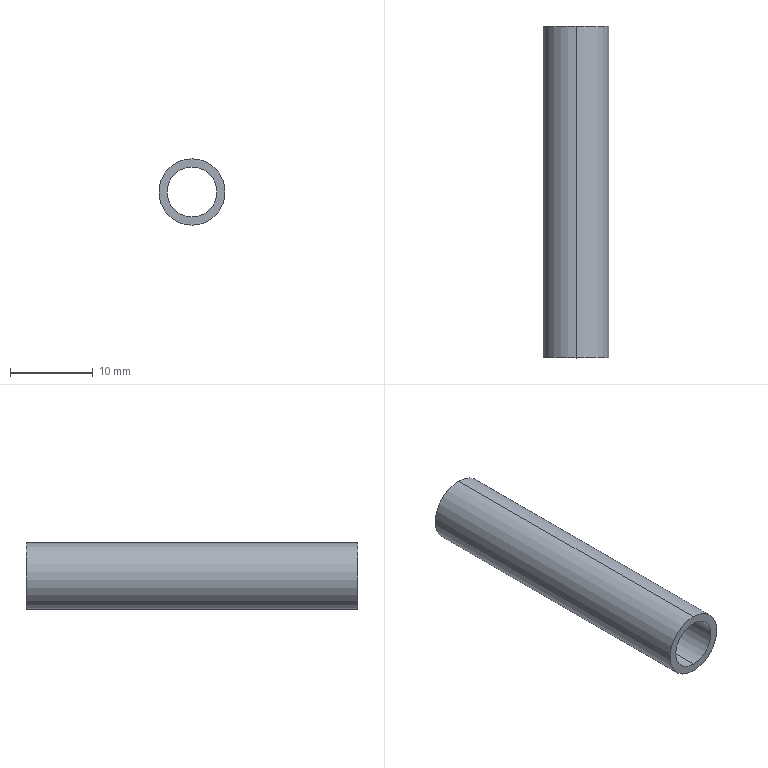Part | SolidWorks | features MirrorStock 1 | 1 solid | 6 faces | box 8 x 40 x 8 mm | volume 879.646 mm3 | cylinder 4 | plane 2 | commonest cylinder face diameters 6 x2 8 x2
STEP:
#1=CARTESIAN_POINT('',(0.,40.,-3.));
#2=VERTEX_POINT('',#1);
#3=CARTESIAN_POINT('',(0.,40.,3.));
#4=VERTEX_POINT('',#3);
#5=CARTESIAN_POINT('',(0.,40.,0.));
#6=DIRECTION('',(0.,-1.,0.));
#7=DIRECTION('',(0.,0.,-1.));
#8=AXIS2_PLACEMENT_3D('',#5,#6,#7);
#9=CIRCLE('',#8,3.);
#10=EDGE_CURVE('',#2,#4,#9,.T.);
#11=ORIENTED_EDGE('',*,*,#10,.F.);
#12=CARTESIAN_POINT('',(0.,0.,-3.));
#13=VERTEX_POINT('',#12);
#14=CARTESIAN_POINT('',(0.,40.,-3.));
#15=DIRECTION('',(0.,-1.,0.));
#16=VECTOR('',#15,1000.);
#17=LINE('',#14,#16);
#18=EDGE_CURVE('',#2,#13,#17,.T.);
#19=ORIENTED_EDGE('',*,*,#18,.T.);
#20=CARTESIAN_POINT('',(0.,0.,3.));
#21=VERTEX_POINT('',#20);
#22=CARTESIAN_POINT('',(0.,0.,0.));
#23=DIRECTION('',(0.,-1.,0.));
#24=DIRECTION('',(0.,0.,-1.));
#25=AXIS2_PLACEMENT_3D('',#22,#23,#24);
#26=CIRCLE('',#25,3.);
#27=EDGE_CURVE('',#13,#21,#26,.T.);
#28=ORIENTED_EDGE('',*,*,#27,.T.);
#29=CARTESIAN_POINT('',(0.,40.,3.));
#30=DIRECTION('',(0.,-1.,0.));
#31=VECTOR('',#30,1000.);
#32=LINE('',#29,#31);
#33=EDGE_CURVE('',#4,#21,#32,.T.);
#34=ORIENTED_EDGE('',*,*,#33,.F.);
#35=EDGE_LOOP('',(#11,#19,#28,#34));
#36=FACE_OUTER_BOUND('',#35,.T.);
#37=CARTESIAN_POINT('',(0.,40.,0.));
#38=DIRECTION('',(0.,-1.,0.));
#39=DIRECTION('',(0.,0.,1.));
#40=AXIS2_PLACEMENT_3D('',#37,#38,#39);
#41=CYLINDRICAL_SURFACE('',#40,3.);
#42=ADVANCED_FACE('',(#36),#41,.F.);
#43=CARTESIAN_POINT('',(0.,40.,4.));
#44=VERTEX_POINT('',#43);
#45=CARTESIAN_POINT('',(0.,40.,-4.));
#46=VERTEX_POINT('',#45);
#47=CARTESIAN_POINT('',(0.,40.,0.));
#48=DIRECTION('',(0.,-1.,0.));
#49=DIRECTION('',(0.,0.,-1.));
#50=AXIS2_PLACEMENT_3D('',#47,#48,#49);
#51=CIRCLE('',#50,4.);
#52=EDGE_CURVE('',#44,#46,#51,.T.);
#53=ORIENTED_EDGE('',*,*,#52,.T.);
#54=CARTESIAN_POINT('',(0.,0.,-4.));
#55=VERTEX_POINT('',#54);
#56=CARTESIAN_POINT('',(0.,40.,-4.));
#57=DIRECTION('',(0.,-1.,0.));
#58=VECTOR('',#57,1000.);
#59=LINE('',#56,#58);
#60=EDGE_CURVE('',#46,#55,#59,.T.);
#61=ORIENTED_EDGE('',*,*,#60,.T.);
#62=CARTESIAN_POINT('',(0.,0.,4.));
#63=VERTEX_POINT('',#62);
#64=CARTESIAN_POINT('',(0.,0.,0.));
#65=DIRECTION('',(0.,-1.,0.));
#66=DIRECTION('',(0.,0.,-1.));
#67=AXIS2_PLACEMENT_3D('',#64,#65,#66);
#68=CIRCLE('',#67,4.);
#69=EDGE_CURVE('',#63,#55,#68,.T.);
#70=ORIENTED_EDGE('',*,*,#69,.F.);
#71=CARTESIAN_POINT('',(0.,40.,4.));
#72=DIRECTION('',(0.,-1.,0.));
#73=VECTOR('',#72,1000.);
#74=LINE('',#71,#73);
#75=EDGE_CURVE('',#44,#63,#74,.T.);
#76=ORIENTED_EDGE('',*,*,#75,.F.);
#77=EDGE_LOOP('',(#53,#61,#70,#76));
#78=FACE_OUTER_BOUND('',#77,.T.);
#79=CARTESIAN_POINT('',(0.,40.,0.));
#80=DIRECTION('',(0.,-1.,0.));
#81=DIRECTION('',(0.,0.,1.));
#82=AXIS2_PLACEMENT_3D('',#79,#80,#81);
#83=CYLINDRICAL_SURFACE('',#82,4.);
#84=ADVANCED_FACE('',(#78),#83,.T.);
#85=ORIENTED_EDGE('',*,*,#52,.F.);
#86=CARTESIAN_POINT('',(0.,40.,0.));
#87=DIRECTION('',(0.,-1.,0.));
#88=DIRECTION('',(0.,0.,-1.));
#89=AXIS2_PLACEMENT_3D('',#86,#87,#88);
#90=CIRCLE('',#89,4.);
#91=EDGE_CURVE('',#46,#44,#90,.T.);
#92=ORIENTED_EDGE('',*,*,#91,.F.);
#93=EDGE_LOOP('',(#85,#92));
#94=FACE_OUTER_BOUND('',#93,.T.);
#95=CARTESIAN_POINT('',(0.,40.,0.));
#96=DIRECTION('',(0.,-1.,0.));
#97=DIRECTION('',(0.,0.,-1.));
#98=AXIS2_PLACEMENT_3D('',#95,#96,#97);
#99=CIRCLE('',#98,3.);
#100=EDGE_CURVE('',#4,#2,#99,.T.);
#101=ORIENTED_EDGE('',*,*,#100,.T.);
#102=ORIENTED_EDGE('',*,*,#10,.T.);
#103=EDGE_LOOP('',(#101,#102));
#104=FACE_BOUND('',#103,.T.);
#105=CARTESIAN_POINT('',(0.,40.,0.));
#106=DIRECTION('',(0.,1.,0.));
#107=DIRECTION('',(0.,0.,-1.));
#108=AXIS2_PLACEMENT_3D('',#105,#106,#107);
#109=PLANE('',#108);
#110=ADVANCED_FACE('',(#94,#104),#109,.T.);
#111=ORIENTED_EDGE('',*,*,#69,.T.);
#112=CARTESIAN_POINT('',(0.,0.,0.));
#113=DIRECTION('',(0.,-1.,0.));
#114=DIRECTION('',(0.,0.,-1.));
#115=AXIS2_PLACEMENT_3D('',#112,#113,#114);
#116=CIRCLE('',#115,4.);
#117=EDGE_CURVE('',#55,#63,#116,.T.);
#118=ORIENTED_EDGE('',*,*,#117,.T.);
#119=EDGE_LOOP('',(#111,#118));
#120=FACE_OUTER_BOUND('',#119,.T.);
#121=CARTESIAN_POINT('',(0.,0.,0.));
#122=DIRECTION('',(0.,-1.,0.));
#123=DIRECTION('',(0.,0.,-1.));
#124=AXIS2_PLACEMENT_3D('',#121,#122,#123);
#125=CIRCLE('',#124,3.);
#126=EDGE_CURVE('',#21,#13,#125,.T.);
#127=ORIENTED_EDGE('',*,*,#126,.F.);
#128=ORIENTED_EDGE('',*,*,#27,.F.);
#129=EDGE_LOOP('',(#127,#128));
#130=FACE_BOUND('',#129,.T.);
#131=CARTESIAN_POINT('',(0.,0.,0.));
#132=DIRECTION('',(0.,1.,0.));
#133=DIRECTION('',(0.,0.,-1.));
#134=AXIS2_PLACEMENT_3D('',#131,#132,#133);
#135=PLANE('',#134);
#136=ADVANCED_FACE('',(#120,#130),#135,.F.);
#137=ORIENTED_EDGE('',*,*,#60,.F.);
#138=ORIENTED_EDGE('',*,*,#91,.T.);
#139=ORIENTED_EDGE('',*,*,#75,.T.);
#140=ORIENTED_EDGE('',*,*,#117,.F.);
#141=EDGE_LOOP('',(#137,#138,#139,#140));
#142=FACE_OUTER_BOUND('',#141,.T.);
#143=CARTESIAN_POINT('',(0.,40.,0.));
#144=DIRECTION('',(0.,-1.,0.));
#145=DIRECTION('',(0.,0.,1.));
#146=AXIS2_PLACEMENT_3D('',#143,#144,#145);
#147=CYLINDRICAL_SURFACE('',#146,4.);
#148=ADVANCED_FACE('',(#142),#147,.T.);
#149=ORIENTED_EDGE('',*,*,#18,.F.);
#150=ORIENTED_EDGE('',*,*,#100,.F.);
#151=ORIENTED_EDGE('',*,*,#33,.T.);
#152=ORIENTED_EDGE('',*,*,#126,.T.);
#153=EDGE_LOOP('',(#149,#150,#151,#152));
#154=FACE_OUTER_BOUND('',#153,.T.);
#155=CARTESIAN_POINT('',(0.,40.,0.));
#156=DIRECTION('',(0.,-1.,0.));
#157=DIRECTION('',(0.,0.,1.));
#158=AXIS2_PLACEMENT_3D('',#155,#156,#157);
#159=CYLINDRICAL_SURFACE('',#158,3.);
#160=ADVANCED_FACE('',(#154),#159,.F.);
#161=CLOSED_SHELL('',(#42,#84,#110,#136,#148,#160));
#162=MANIFOLD_SOLID_BREP('',#161);
#163=CARTESIAN_POINT('',(0.,0.,0.));
#164=DIRECTION('',(0.,0.,1.));
#165=DIRECTION('',(1.,0.,0.));
#166=AXIS2_PLACEMENT_3D('',#163,#164,#165);
#167=(LENGTH_UNIT()NAMED_UNIT(*)SI_UNIT(.MILLI.,.METRE.));
#168=UNCERTAINTY_MEASURE_WITH_UNIT(LENGTH_MEASURE(0.00001),#167,'','');
#169=(NAMED_UNIT(*)PLANE_ANGLE_UNIT()SI_UNIT($,.RADIAN.));
#170=(NAMED_UNIT(*)SI_UNIT($,.STERADIAN.)SOLID_ANGLE_UNIT());
#171=(GEOMETRIC_REPRESENTATION_CONTEXT(3)GLOBAL_UNCERTAINTY_ASSIGNED_CONTEXT((#168))GLOBAL_UNIT_ASSIGNED_CONTEXT((#167,#169,#170))REPRESENTATION_CONTEXT('',''));
#172=ADVANCED_BREP_SHAPE_REPRESENTATION('',(#162,#166),#171);